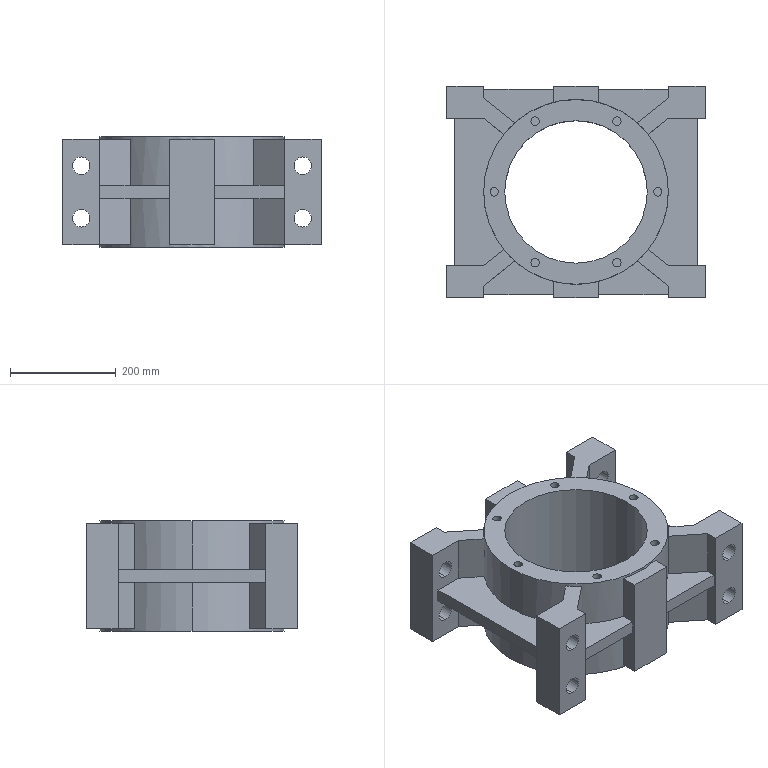Part | NX | features DATUM_CSYS 2, SKETCH 2, BREP 1 | 1 solid | 128 faces | box 490 x 400 x 210 mm | volume 14928889 mm3 | plane 82 | cylinder 46 | commonest cylinder face diameters 16 x24 33 x16 350 x4 270 x2